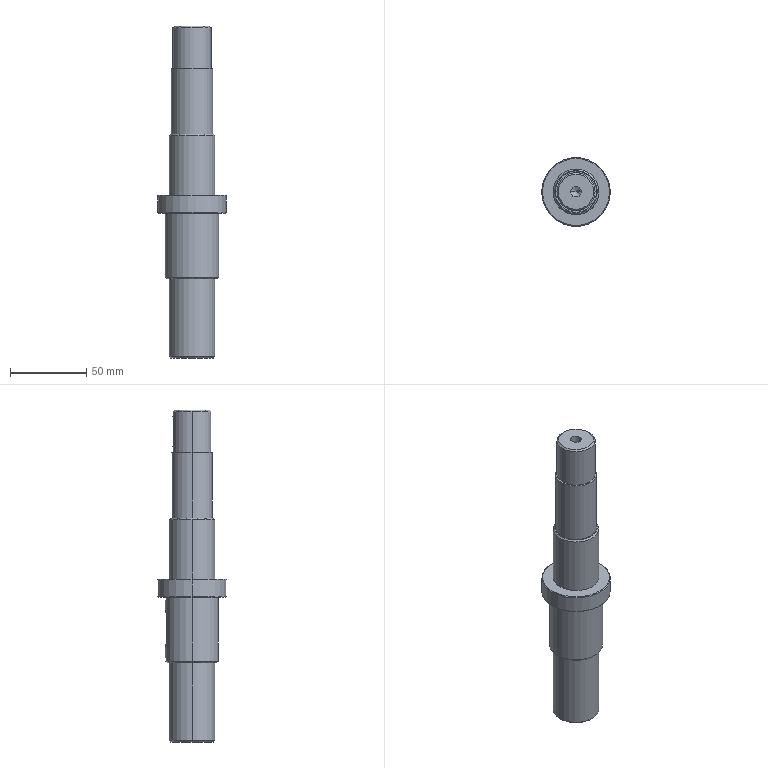Part | SolidWorks | features ICE 7, Chamfer 3, 3DProfileFeature 1, Extrusion 1, HoleWzd 1 | 1 solid | 47 faces | box 45 x 45 x 218 mm | volume 161225 mm3 | cylinder 20 | cone 14 | plane 13 | commonest cylinder face diameters 30 x4 8 x3 10 x3 7 x2 25 x2 27 x2
STEP:
#1=CARTESIAN_POINT('',(-3.5,0.,199.));
#2=VERTEX_POINT('',#1);
#3=CARTESIAN_POINT('',(3.5,0.,199.));
#4=VERTEX_POINT('',#3);
#5=CARTESIAN_POINT('',(0.,0.,199.));
#6=DIRECTION('',(0.,0.,1.));
#7=DIRECTION('',(1.,0.,0.));
#8=AXIS2_PLACEMENT_3D('',#5,#6,#7);
#9=CIRCLE('',#8,3.5);
#10=EDGE_CURVE('',#2,#4,#9,.T.);
#11=ORIENTED_EDGE('',*,*,#10,.F.);
#12=CARTESIAN_POINT('',(-3.5,0.,218.));
#13=VERTEX_POINT('',#12);
#14=CARTESIAN_POINT('',(-3.5,0.,218.));
#15=DIRECTION('',(0.,0.,1.));
#16=VECTOR('',#15,1000.);
#17=LINE('',#14,#16);
#18=EDGE_CURVE('',#2,#13,#17,.T.);
#19=ORIENTED_EDGE('',*,*,#18,.T.);
#20=CARTESIAN_POINT('',(3.5,0.,218.));
#21=VERTEX_POINT('',#20);
#22=CARTESIAN_POINT('',(0.,0.,218.));
#23=DIRECTION('',(0.,0.,1.));
#24=DIRECTION('',(1.,0.,0.));
#25=AXIS2_PLACEMENT_3D('',#22,#23,#24);
#26=CIRCLE('',#25,3.5);
#27=EDGE_CURVE('',#13,#21,#26,.T.);
#28=ORIENTED_EDGE('',*,*,#27,.T.);
#29=CARTESIAN_POINT('',(3.5,0.,218.));
#30=DIRECTION('',(0.,0.,1.));
#31=VECTOR('',#30,1000.);
#32=LINE('',#29,#31);
#33=EDGE_CURVE('',#4,#21,#32,.T.);
#34=ORIENTED_EDGE('',*,*,#33,.F.);
#35=EDGE_LOOP('',(#11,#19,#28,#34));
#36=FACE_OUTER_BOUND('',#35,.T.);
#37=CARTESIAN_POINT('',(0.,0.,218.));
#38=DIRECTION('',(0.,0.,1.));
#39=DIRECTION('',(1.,0.,0.));
#40=AXIS2_PLACEMENT_3D('',#37,#38,#39);
#41=CYLINDRICAL_SURFACE('',#40,3.5);
#42=ADVANCED_FACE('',(#36),#41,.F.);
#43=CARTESIAN_POINT('',(0.,0.,196.897));
#44=VERTEX_POINT('',#43);
#45=CARTESIAN_POINT('',(3.5,0.,199.));
#46=DIRECTION('',(0.8572,0.,0.515));
#47=VECTOR('',#46,1000.);
#48=LINE('',#45,#47);
#49=EDGE_CURVE('',#44,#4,#48,.T.);
#50=ORIENTED_EDGE('',*,*,#49,.F.);
#51=CARTESIAN_POINT('',(-3.5,0.,199.));
#52=DIRECTION('',(-0.8572,0.,0.515));
#53=VECTOR('',#52,1000.);
#54=LINE('',#51,#53);
#55=EDGE_CURVE('',#44,#2,#54,.T.);
#56=ORIENTED_EDGE('',*,*,#55,.T.);
#57=ORIENTED_EDGE('',*,*,#10,.T.);
#58=EDGE_LOOP('',(#50,#56,#57));
#59=FACE_OUTER_BOUND('',#58,.T.);
#60=CARTESIAN_POINT('',(0.,0.,199.));
#61=DIRECTION('',(0.,0.,1.));
#62=DIRECTION('',(1.,0.,0.));
#63=AXIS2_PLACEMENT_3D('',#60,#61,#62);
#64=CONICAL_SURFACE('',#63,3.5,1.03);
#65=ADVANCED_FACE('',(#59),#64,.F.);
#66=CARTESIAN_POINT('',(4.,11.843,198.));
#67=VERTEX_POINT('',#66);
#68=CARTESIAN_POINT('',(0.,12.5,194.));
#69=VERTEX_POINT('',#68);
#70=CARTESIAN_POINT('',(4.,11.843,198.));
#71=CARTESIAN_POINT('',(4.,11.843,197.734));
#72=CARTESIAN_POINT('',(3.974,11.852,197.472));
#73=CARTESIAN_POINT('',(3.871,11.886,196.959));
#74=CARTESIAN_POINT('',(3.793,11.911,196.704));
#75=CARTESIAN_POINT('',(3.592,11.973,196.22));
#76=CARTESIAN_POINT('',(3.469,12.01,195.991));
#77=CARTESIAN_POINT('',(3.178,12.09,195.557));
#78=CARTESIAN_POINT('',(3.011,12.134,195.354));
#79=CARTESIAN_POINT('',(2.644,12.219,194.987));
#80=CARTESIAN_POINT('',(2.444,12.261,194.822));
#81=CARTESIAN_POINT('',(2.006,12.34,194.53));
#82=CARTESIAN_POINT('',(1.776,12.375,194.407));
#83=CARTESIAN_POINT('',(1.295,12.435,194.207));
#84=CARTESIAN_POINT('',(1.041,12.459,194.129));
#85=CARTESIAN_POINT('',(0.5239,12.492,194.026));
#86=CARTESIAN_POINT('',(0.263,12.5,194.));
#87=CARTESIAN_POINT('',(0.,12.5,194.));
#88=B_SPLINE_CURVE_WITH_KNOTS('',3,(#70,#71,#72,#73,#74,#75,#76,#77,#78,#79,#80,#81,#82,#83,#84,#85,#86,#87),.UNSPECIFIED.,.F.,.F.,(4,2,2,2,2,2,2,2,4),(0.,0.000787,0.001574,0.002361,0.003148,0.003935,0.004722,0.005509,0.006296),.UNSPECIFIED.);
#89=EDGE_CURVE('',#67,#69,#88,.T.);
#90=ORIENTED_EDGE('',*,*,#89,.T.);
#91=CARTESIAN_POINT('',(0.,8.5,194.));
#92=VERTEX_POINT('',#91);
#93=CARTESIAN_POINT('',(0.,18.5,194.));
#94=DIRECTION('',(0.,-1.,0.));
#95=VECTOR('',#94,1000.);
#96=LINE('',#93,#95);
#97=EDGE_CURVE('',#69,#92,#96,.T.);
#98=ORIENTED_EDGE('',*,*,#97,.T.);
#99=CARTESIAN_POINT('',(4.,8.5,198.));
#100=VERTEX_POINT('',#99);
#101=CARTESIAN_POINT('',(0.,8.5,198.));
#102=DIRECTION('',(0.,1.,0.));
#103=DIRECTION('',(0.,0.,1.));
#104=AXIS2_PLACEMENT_3D('',#101,#102,#103);
#105=CIRCLE('',#104,4.);
#106=EDGE_CURVE('',#100,#92,#105,.T.);
#107=ORIENTED_EDGE('',*,*,#106,.F.);
#108=CARTESIAN_POINT('',(4.,18.5,198.));
#109=DIRECTION('',(0.,-1.,0.));
#110=VECTOR('',#109,1000.);
#111=LINE('',#108,#110);
#112=EDGE_CURVE('',#67,#100,#111,.T.);
#113=ORIENTED_EDGE('',*,*,#112,.F.);
#114=EDGE_LOOP('',(#90,#98,#107,#113));
#115=FACE_OUTER_BOUND('',#114,.T.);
#116=CARTESIAN_POINT('',(0.,18.5,198.));
#117=DIRECTION('',(0.,-1.,0.));
#118=DIRECTION('',(0.,0.,-1.));
#119=AXIS2_PLACEMENT_3D('',#116,#117,#118);
#120=CYLINDRICAL_SURFACE('',#119,4.);
#121=ADVANCED_FACE('',(#115),#120,.F.);
#122=CARTESIAN_POINT('',(5.,16.771,67.));
#123=VERTEX_POINT('',#122);
#124=CARTESIAN_POINT('',(0.,17.5,62.));
#125=VERTEX_POINT('',#124);
#126=CARTESIAN_POINT('',(5.,16.771,67.));
#127=CARTESIAN_POINT('',(5.,16.771,66.668));
#128=CARTESIAN_POINT('',(4.967,16.78,66.341));
#129=CARTESIAN_POINT('',(4.839,16.818,65.7));
#130=CARTESIAN_POINT('',(4.742,16.846,65.381));
#131=CARTESIAN_POINT('',(4.49,16.915,64.776));
#132=CARTESIAN_POINT('',(4.337,16.955,64.49));
#133=CARTESIAN_POINT('',(3.974,17.044,63.948));
#134=CARTESIAN_POINT('',(3.764,17.092,63.692));
#135=CARTESIAN_POINT('',(3.305,17.187,63.234));
#136=CARTESIAN_POINT('',(3.054,17.234,63.027));
#137=CARTESIAN_POINT('',(2.507,17.322,62.662));
#138=CARTESIAN_POINT('',(2.219,17.361,62.508));
#139=CARTESIAN_POINT('',(1.768,17.411,62.32));
#140=CARTESIAN_POINT('',(1.614,17.426,62.265));
#141=CARTESIAN_POINT('',(1.3,17.452,62.169));
#142=CARTESIAN_POINT('',(1.139,17.464,62.129));
#143=CARTESIAN_POINT('',(0.6539,17.491,62.032));
#144=CARTESIAN_POINT('',(0.3282,17.5,62.));
#145=CARTESIAN_POINT('',(0.,17.5,62.));
#146=B_SPLINE_CURVE_WITH_KNOTS('',3,(#126,#127,#128,#129,#130,#131,#132,#133,#134,#135,#136,#137,#138,#139,#140,#141,#142,#143,#144,#145),.UNSPECIFIED.,.F.,.F.,(4,2,2,2,2,2,2,2,2,4),(0.,0.0009824,0.001965,0.002947,0.00393,0.004912,0.005894,0.006386,0.006877,0.007859),.UNSPECIFIED.);
#147=EDGE_CURVE('',#123,#125,#146,.T.);
#148=ORIENTED_EDGE('',*,*,#147,.T.);
#149=CARTESIAN_POINT('',(0.,12.5,62.));
#150=VERTEX_POINT('',#149);
#151=CARTESIAN_POINT('',(0.,32.5,62.));
#152=DIRECTION('',(0.,-1.,0.));
#153=VECTOR('',#152,1000.);
#154=LINE('',#151,#153);
#155=EDGE_CURVE('',#125,#150,#154,.T.);
#156=ORIENTED_EDGE('',*,*,#155,.T.);
#157=CARTESIAN_POINT('',(5.,12.5,67.));
#158=VERTEX_POINT('',#157);
#159=CARTESIAN_POINT('',(0.,12.5,67.));
#160=DIRECTION('',(0.,1.,0.));
#161=DIRECTION('',(0.,0.,1.));
#162=AXIS2_PLACEMENT_3D('',#159,#160,#161);
#163=CIRCLE('',#162,5.);
#164=EDGE_CURVE('',#158,#150,#163,.T.);
#165=ORIENTED_EDGE('',*,*,#164,.F.);
#166=CARTESIAN_POINT('',(5.,32.5,67.));
#167=DIRECTION('',(0.,-1.,0.));
#168=VECTOR('',#167,1000.);
#169=LINE('',#166,#168);
#170=EDGE_CURVE('',#123,#158,#169,.T.);
#171=ORIENTED_EDGE('',*,*,#170,.F.);
#172=EDGE_LOOP('',(#148,#156,#165,#171));
#173=FACE_OUTER_BOUND('',#172,.T.);
#174=CARTESIAN_POINT('',(0.,32.5,67.));
#175=DIRECTION('',(0.,-1.,0.));
#176=DIRECTION('',(0.,0.,-1.));
#177=AXIS2_PLACEMENT_3D('',#174,#175,#176);
#178=CYLINDRICAL_SURFACE('',#177,5.);
#179=ADVANCED_FACE('',(#173),#178,.F.);
#180=CARTESIAN_POINT('',(-22.,0.,95.));
#181=VERTEX_POINT('',#180);
#182=CARTESIAN_POINT('',(22.,0.,95.));
#183=VERTEX_POINT('',#182);
#184=CARTESIAN_POINT('',(0.,0.,95.));
#185=DIRECTION('',(0.,0.,-1.));
#186=DIRECTION('',(1.,0.,0.));
#187=AXIS2_PLACEMENT_3D('',#184,#185,#186);
#188=CIRCLE('',#187,22.);
#189=EDGE_CURVE('',#181,#183,#188,.T.);
#190=ORIENTED_EDGE('',*,*,#189,.F.);
#191=CARTESIAN_POINT('',(-22.5,0.,95.5));
#192=VERTEX_POINT('',#191);
#193=CARTESIAN_POINT('',(-22.5,0.,95.5));
#194=DIRECTION('',(-0.7071,0.,0.7071));
#195=VECTOR('',#194,1000.);
#196=LINE('',#193,#195);
#197=EDGE_CURVE('',#181,#192,#196,.T.);
#198=ORIENTED_EDGE('',*,*,#197,.T.);
#199=CARTESIAN_POINT('',(22.5,0.,95.5));
#200=VERTEX_POINT('',#199);
#201=CARTESIAN_POINT('',(0.,0.,95.5));
#202=DIRECTION('',(0.,0.,1.));
#203=DIRECTION('',(1.,0.,0.));
#204=AXIS2_PLACEMENT_3D('',#201,#202,#203);
#205=CIRCLE('',#204,22.5);
#206=EDGE_CURVE('',#200,#192,#205,.T.);
#207=ORIENTED_EDGE('',*,*,#206,.F.);
#208=CARTESIAN_POINT('',(22.5,0.,95.5));
#209=DIRECTION('',(0.7071,0.,0.7071));
#210=VECTOR('',#209,1000.);
#211=LINE('',#208,#210);
#212=EDGE_CURVE('',#183,#200,#211,.T.);
#213=ORIENTED_EDGE('',*,*,#212,.F.);
#214=EDGE_LOOP('',(#190,#198,#207,#213));
#215=FACE_OUTER_BOUND('',#214,.T.);
#216=CARTESIAN_POINT('',(0.,0.,95.5));
#217=DIRECTION('',(0.,0.,1.));
#218=DIRECTION('',(1.,0.,0.));
#219=AXIS2_PLACEMENT_3D('',#216,#217,#218);
#220=CONICAL_SURFACE('',#219,22.5,0.7854);
#221=ADVANCED_FACE('',(#215),#220,.T.);
#222=CARTESIAN_POINT('',(22.,0.,107.));
#223=VERTEX_POINT('',#222);
#224=CARTESIAN_POINT('',(-22.,0.,107.));
#225=VERTEX_POINT('',#224);
#226=CARTESIAN_POINT('',(0.,0.,107.));
#227=DIRECTION('',(0.,0.,1.));
#228=DIRECTION('',(1.,0.,0.));
#229=AXIS2_PLACEMENT_3D('',#226,#227,#228);
#230=CIRCLE('',#229,22.);
#231=EDGE_CURVE('',#223,#225,#230,.T.);
#232=ORIENTED_EDGE('',*,*,#231,.F.);
#233=CARTESIAN_POINT('',(22.5,0.,106.5));
#234=VERTEX_POINT('',#233);
#235=CARTESIAN_POINT('',(22.,0.,107.));
#236=DIRECTION('',(0.7071,0.,-0.7071));
#237=VECTOR('',#236,1000.);
#238=LINE('',#235,#237);
#239=EDGE_CURVE('',#223,#234,#238,.T.);
#240=ORIENTED_EDGE('',*,*,#239,.T.);
#241=CARTESIAN_POINT('',(-22.5,0.,106.5));
#242=VERTEX_POINT('',#241);
#243=CARTESIAN_POINT('',(0.,0.,106.5));
#244=DIRECTION('',(0.,0.,-1.));
#245=DIRECTION('',(1.,0.,0.));
#246=AXIS2_PLACEMENT_3D('',#243,#244,#245);
#247=CIRCLE('',#246,22.5);
#248=EDGE_CURVE('',#242,#234,#247,.T.);
#249=ORIENTED_EDGE('',*,*,#248,.F.);
#250=CARTESIAN_POINT('',(-22.,0.,107.));
#251=DIRECTION('',(-0.7071,0.,-0.7071));
#252=VECTOR('',#251,1000.);
#253=LINE('',#250,#252);
#254=EDGE_CURVE('',#225,#242,#253,.T.);
#255=ORIENTED_EDGE('',*,*,#254,.F.);
#256=EDGE_LOOP('',(#232,#240,#249,#255));
#257=FACE_OUTER_BOUND('',#256,.T.);
#258=CARTESIAN_POINT('',(0.,0.,107.));
#259=DIRECTION('',(0.,0.,-1.));
#260=DIRECTION('',(-1.,0.,0.));
#261=AXIS2_PLACEMENT_3D('',#258,#259,#260);
#262=CONICAL_SURFACE('',#261,22.,0.7854);
#263=ADVANCED_FACE('',(#257),#262,.T.);
#264=CARTESIAN_POINT('',(-16.5,0.,52.));
#265=VERTEX_POINT('',#264);
#266=CARTESIAN_POINT('',(16.5,0.,52.));
#267=VERTEX_POINT('',#266);
#268=CARTESIAN_POINT('',(0.,0.,52.));
#269=DIRECTION('',(0.,0.,-1.));
#270=DIRECTION('',(1.,0.,0.));
#271=AXIS2_PLACEMENT_3D('',#268,#269,#270);
#272=CIRCLE('',#271,16.5);
#273=EDGE_CURVE('',#265,#267,#272,.T.);
#274=ORIENTED_EDGE('',*,*,#273,.F.);
#275=CARTESIAN_POINT('',(-17.5,0.,53.));
#276=VERTEX_POINT('',#275);
#277=CARTESIAN_POINT('',(-17.5,0.,53.));
#278=DIRECTION('',(-0.7071,0.,0.7071));
#279=VECTOR('',#278,1000.);
#280=LINE('',#277,#279);
#281=EDGE_CURVE('',#265,#276,#280,.T.);
#282=ORIENTED_EDGE('',*,*,#281,.T.);
#283=CARTESIAN_POINT('',(17.5,0.,53.));
#284=VERTEX_POINT('',#283);
#285=CARTESIAN_POINT('',(0.,0.,53.));
#286=DIRECTION('',(0.,0.,1.));
#287=DIRECTION('',(1.,0.,0.));
#288=AXIS2_PLACEMENT_3D('',#285,#286,#287);
#289=CIRCLE('',#288,17.5);
#290=EDGE_CURVE('',#284,#276,#289,.T.);
#291=ORIENTED_EDGE('',*,*,#290,.F.);
#292=CARTESIAN_POINT('',(17.5,0.,53.));
#293=DIRECTION('',(0.7071,0.,0.7071));
#294=VECTOR('',#293,1000.);
#295=LINE('',#292,#294);
#296=EDGE_CURVE('',#267,#284,#295,.T.);
#297=ORIENTED_EDGE('',*,*,#296,.F.);
#298=EDGE_LOOP('',(#274,#282,#291,#297));
#299=FACE_OUTER_BOUND('',#298,.T.);
#300=CARTESIAN_POINT('',(0.,0.,53.));
#301=DIRECTION('',(0.,0.,1.));
#302=DIRECTION('',(1.,0.,0.));
#303=AXIS2_PLACEMENT_3D('',#300,#301,#302);
#304=CONICAL_SURFACE('',#303,17.5,0.7854);
#305=ADVANCED_FACE('',(#299),#304,.T.);
#306=CARTESIAN_POINT('',(14.,0.,147.));
#307=VERTEX_POINT('',#306);
#308=CARTESIAN_POINT('',(-14.,0.,147.));
#309=VERTEX_POINT('',#308);
#310=CARTESIAN_POINT('',(0.,0.,147.));
#311=DIRECTION('',(0.,0.,1.));
#312=DIRECTION('',(1.,0.,0.));
#313=AXIS2_PLACEMENT_3D('',#310,#311,#312);
#314=CIRCLE('',#313,14.);
#315=EDGE_CURVE('',#307,#309,#314,.T.);
#316=ORIENTED_EDGE('',*,*,#315,.F.);
#317=CARTESIAN_POINT('',(15.,0.,146.));
#318=VERTEX_POINT('',#317);
#319=CARTESIAN_POINT('',(14.,0.,147.));
#320=DIRECTION('',(0.7071,0.,-0.7071));
#321=VECTOR('',#320,1000.);
#322=LINE('',#319,#321);
#323=EDGE_CURVE('',#307,#318,#322,.T.);
#324=ORIENTED_EDGE('',*,*,#323,.T.);
#325=CARTESIAN_POINT('',(-15.,0.,146.));
#326=VERTEX_POINT('',#325);
#327=CARTESIAN_POINT('',(0.,0.,146.));
#328=DIRECTION('',(0.,0.,-1.));
#329=DIRECTION('',(1.,0.,0.));
#330=AXIS2_PLACEMENT_3D('',#327,#328,#329);
#331=CIRCLE('',#330,15.);
#332=EDGE_CURVE('',#326,#318,#331,.T.);
#333=ORIENTED_EDGE('',*,*,#332,.F.);
#334=CARTESIAN_POINT('',(-14.,0.,147.));
#335=DIRECTION('',(-0.7071,0.,-0.7071));
#336=VECTOR('',#335,1000.);
#337=LINE('',#334,#336);
#338=EDGE_CURVE('',#309,#326,#337,.T.);
#339=ORIENTED_EDGE('',*,*,#338,.F.);
#340=EDGE_LOOP('',(#316,#324,#333,#339));
#341=FACE_OUTER_BOUND('',#340,.T.);
#342=CARTESIAN_POINT('',(0.,0.,147.));
#343=DIRECTION('',(0.,0.,-1.));
#344=DIRECTION('',(-1.,0.,0.));
#345=AXIS2_PLACEMENT_3D('',#342,#343,#344);
#346=CONICAL_SURFACE('',#345,14.,0.7854);
#347=ADVANCED_FACE('',(#341),#346,.T.);
#348=CARTESIAN_POINT('',(11.5,0.,218.));
#349=VERTEX_POINT('',#348);
#350=CARTESIAN_POINT('',(-11.5,0.,218.));
#351=VERTEX_POINT('',#350);
#352=CARTESIAN_POINT('',(0.,0.,218.));
#353=DIRECTION('',(0.,0.,1.));
#354=DIRECTION('',(1.,0.,0.));
#355=AXIS2_PLACEMENT_3D('',#352,#353,#354);
#356=CIRCLE('',#355,11.5);
#357=EDGE_CURVE('',#349,#351,#356,.T.);
#358=ORIENTED_EDGE('',*,*,#357,.F.);
#359=CARTESIAN_POINT('',(12.5,0.,217.));
#360=VERTEX_POINT('',#359);
#361=CARTESIAN_POINT('',(11.5,0.,218.));
#362=DIRECTION('',(0.7071,0.,-0.7071));
#363=VECTOR('',#362,1000.);
#364=LINE('',#361,#363);
#365=EDGE_CURVE('',#349,#360,#364,.T.);
#366=ORIENTED_EDGE('',*,*,#365,.T.);
#367=CARTESIAN_POINT('',(-12.5,0.,217.));
#368=VERTEX_POINT('',#367);
#369=CARTESIAN_POINT('',(0.,0.,217.));
#370=DIRECTION('',(0.,0.,-1.));
#371=DIRECTION('',(1.,0.,0.));
#372=AXIS2_PLACEMENT_3D('',#369,#370,#371);
#373=CIRCLE('',#372,12.5);
#374=EDGE_CURVE('',#368,#360,#373,.T.);
#375=ORIENTED_EDGE('',*,*,#374,.F.);
#376=CARTESIAN_POINT('',(-11.5,0.,218.));
#377=DIRECTION('',(-0.7071,0.,-0.7071));
#378=VECTOR('',#377,1000.);
#379=LINE('',#376,#378);
#380=EDGE_CURVE('',#351,#368,#379,.T.);
#381=ORIENTED_EDGE('',*,*,#380,.F.);
#382=EDGE_LOOP('',(#358,#366,#375,#381));
#383=FACE_OUTER_BOUND('',#382,.T.);
#384=CARTESIAN_POINT('',(0.,0.,218.));
#385=DIRECTION('',(0.,0.,-1.));
#386=DIRECTION('',(-1.,0.,0.));
#387=AXIS2_PLACEMENT_3D('',#384,#385,#386);
#388=CONICAL_SURFACE('',#387,11.5,0.7854);
#389=ADVANCED_FACE('',(#383),#388,.T.);
#390=CARTESIAN_POINT('',(-14.,0.,0.));
#391=VERTEX_POINT('',#390);
#392=CARTESIAN_POINT('',(14.,0.,0.));
#393=VERTEX_POINT('',#392);
#394=CARTESIAN_POINT('',(0.,0.,0.));
#395=DIRECTION('',(0.,0.,-1.));
#396=DIRECTION('',(1.,0.,0.));
#397=AXIS2_PLACEMENT_3D('',#394,#395,#396);
#398=CIRCLE('',#397,14.);
#399=EDGE_CURVE('',#391,#393,#398,.T.);
#400=ORIENTED_EDGE('',*,*,#399,.F.);
#401=CARTESIAN_POINT('',(-15.,0.,1.));
#402=VERTEX_POINT('',#401);
#403=CARTESIAN_POINT('',(-15.,0.,1.));
#404=DIRECTION('',(-0.7071,0.,0.7071));
#405=VECTOR('',#404,1000.);
#406=LINE('',#403,#405);
#407=EDGE_CURVE('',#391,#402,#406,.T.);
#408=ORIENTED_EDGE('',*,*,#407,.T.);
#409=CARTESIAN_POINT('',(15.,0.,1.));
#410=VERTEX_POINT('',#409);
#411=CARTESIAN_POINT('',(0.,0.,1.));
#412=DIRECTION('',(0.,0.,1.));
#413=DIRECTION('',(1.,0.,0.));
#414=AXIS2_PLACEMENT_3D('',#411,#412,#413);
#415=CIRCLE('',#414,15.);
#416=EDGE_CURVE('',#410,#402,#415,.T.);
#417=ORIENTED_EDGE('',*,*,#416,.F.);
#418=CARTESIAN_POINT('',(15.,0.,1.));
#419=DIRECTION('',(0.7071,0.,0.7071));
#420=VECTOR('',#419,1000.);
#421=LINE('',#418,#420);
#422=EDGE_CURVE('',#393,#410,#421,.T.);
#423=ORIENTED_EDGE('',*,*,#422,.F.);
#424=EDGE_LOOP('',(#400,#408,#417,#423));
#425=FACE_OUTER_BOUND('',#424,.T.);
#426=CARTESIAN_POINT('',(0.,0.,1.));
#427=DIRECTION('',(0.,0.,1.));
#428=DIRECTION('',(1.,0.,0.));
#429=AXIS2_PLACEMENT_3D('',#426,#427,#428);
#430=CONICAL_SURFACE('',#429,15.,0.7854);
#431=ADVANCED_FACE('',(#425),#430,.T.);
#432=CARTESIAN_POINT('',(13.5,0.,190.));
#433=VERTEX_POINT('',#432);
#434=CARTESIAN_POINT('',(-13.5,0.,190.));
#435=VERTEX_POINT('',#434);
#436=CARTESIAN_POINT('',(0.,0.,190.));
#437=DIRECTION('',(0.,0.,1.));
#438=DIRECTION('',(1.,0.,0.));
#439=AXIS2_PLACEMENT_3D('',#436,#437,#438);
#440=CIRCLE('',#439,13.5);
#441=EDGE_CURVE('',#433,#435,#440,.T.);
#442=ORIENTED_EDGE('',*,*,#441,.F.);
#443=CARTESIAN_POINT('',(13.5,0.,147.));
#444=VERTEX_POINT('',#443);
#445=CARTESIAN_POINT('',(13.5,0.,190.));
#446=DIRECTION('',(0.,0.,-1.));
#447=VECTOR('',#446,1000.);
#448=LINE('',#445,#447);
#449=EDGE_CURVE('',#433,#444,#448,.T.);
#450=ORIENTED_EDGE('',*,*,#449,.T.);
#451=CARTESIAN_POINT('',(-13.5,0.,147.));
#452=VERTEX_POINT('',#451);
#453=CARTESIAN_POINT('',(0.,0.,147.));
#454=DIRECTION('',(0.,0.,1.));
#455=DIRECTION('',(1.,0.,0.));
#456=AXIS2_PLACEMENT_3D('',#453,#454,#455);
#457=CIRCLE('',#456,13.5);
#458=EDGE_CURVE('',#444,#452,#457,.T.);
#459=ORIENTED_EDGE('',*,*,#458,.T.);
#460=CARTESIAN_POINT('',(-13.5,0.,190.));
#461=DIRECTION('',(0.,0.,-1.));
#462=VECTOR('',#461,1000.);
#463=LINE('',#460,#462);
#464=EDGE_CURVE('',#435,#452,#463,.T.);
#465=ORIENTED_EDGE('',*,*,#464,.F.);
#466=EDGE_LOOP('',(#442,#450,#459,#465));
#467=FACE_OUTER_BOUND('',#466,.T.);
#468=CARTESIAN_POINT('',(0.,0.,190.));
#469=DIRECTION('',(0.,0.,-1.));
#470=DIRECTION('',(-1.,0.,0.));
#471=AXIS2_PLACEMENT_3D('',#468,#469,#470);
#472=CYLINDRICAL_SURFACE('',#471,13.5);
#473=ADVANCED_FACE('',(#467),#472,.T.);
#474=ORIENTED_EDGE('',*,*,#332,.T.);
#475=CARTESIAN_POINT('',(15.,0.,107.));
#476=VERTEX_POINT('',#475);
#477=CARTESIAN_POINT('',(15.,0.,147.));
#478=DIRECTION('',(0.,0.,-1.));
#479=VECTOR('',#478,1000.);
#480=LINE('',#477,#479);
#481=EDGE_CURVE('',#318,#476,#480,.T.);
#482=ORIENTED_EDGE('',*,*,#481,.T.);
#483=CARTESIAN_POINT('',(-15.,0.,107.));
#484=VERTEX_POINT('',#483);
#485=CARTESIAN_POINT('',(0.,0.,107.));
#486=DIRECTION('',(0.,0.,1.));
#487=DIRECTION('',(1.,0.,0.));
#488=AXIS2_PLACEMENT_3D('',#485,#486,#487);
#489=CIRCLE('',#488,15.);
#490=EDGE_CURVE('',#476,#484,#489,.T.);
#491=ORIENTED_EDGE('',*,*,#490,.T.);
#492=CARTESIAN_POINT('',(-15.,0.,147.));
#493=DIRECTION('',(0.,0.,-1.));
#494=VECTOR('',#493,1000.);
#495=LINE('',#492,#494);
#496=EDGE_CURVE('',#326,#484,#495,.T.);
#497=ORIENTED_EDGE('',*,*,#496,.F.);
#498=EDGE_LOOP('',(#474,#482,#491,#497));
#499=FACE_OUTER_BOUND('',#498,.T.);
#500=CARTESIAN_POINT('',(0.,0.,147.));
#501=DIRECTION('',(0.,0.,-1.));
#502=DIRECTION('',(-1.,0.,0.));
#503=AXIS2_PLACEMENT_3D('',#500,#501,#502);
#504=CYLINDRICAL_SURFACE('',#503,15.);
#505=ADVANCED_FACE('',(#499),#504,.T.);
#506=ORIENTED_EDGE('',*,*,#248,.T.);
#507=CARTESIAN_POINT('',(22.5,0.,107.));
#508=DIRECTION('',(0.,0.,-1.));
#509=VECTOR('',#508,1000.);
#510=LINE('',#507,#509);
#511=EDGE_CURVE('',#234,#200,#510,.T.);
#512=ORIENTED_EDGE('',*,*,#511,.T.);
#513=ORIENTED_EDGE('',*,*,#206,.T.);
#514=CARTESIAN_POINT('',(-22.5,0.,107.));
#515=DIRECTION('',(0.,0.,-1.));
#516=VECTOR('',#515,1000.);
#517=LINE('',#514,#516);
#518=EDGE_CURVE('',#242,#192,#517,.T.);
#519=ORIENTED_EDGE('',*,*,#518,.F.);
#520=EDGE_LOOP('',(#506,#512,#513,#519));
#521=FACE_OUTER_BOUND('',#520,.T.);
#522=CARTESIAN_POINT('',(0.,0.,107.));
#523=DIRECTION('',(0.,0.,-1.));
#524=DIRECTION('',(-1.,0.,0.));
#525=AXIS2_PLACEMENT_3D('',#522,#523,#524);
#526=CYLINDRICAL_SURFACE('',#525,22.5);
#527=ADVANCED_FACE('',(#521),#526,.T.);
#528=CARTESIAN_POINT('',(15.,0.,52.));
#529=VERTEX_POINT('',#528);
#530=CARTESIAN_POINT('',(-15.,0.,52.));
#531=VERTEX_POINT('',#530);
#532=CARTESIAN_POINT('',(0.,0.,52.));
#533=DIRECTION('',(0.,0.,1.));
#534=DIRECTION('',(1.,0.,0.));
#535=AXIS2_PLACEMENT_3D('',#532,#533,#534);
#536=CIRCLE('',#535,15.);
#537=EDGE_CURVE('',#529,#531,#536,.T.);
#538=ORIENTED_EDGE('',*,*,#537,.F.);
#539=CARTESIAN_POINT('',(15.,0.,52.));
#540=DIRECTION('',(0.,0.,-1.));
#541=VECTOR('',#540,1000.);
#542=LINE('',#539,#541);
#543=EDGE_CURVE('',#529,#410,#542,.T.);
#544=ORIENTED_EDGE('',*,*,#543,.T.);
#545=ORIENTED_EDGE('',*,*,#416,.T.);
#546=CARTESIAN_POINT('',(-15.,0.,52.));
#547=DIRECTION('',(0.,0.,-1.));
#548=VECTOR('',#547,1000.);
#549=LINE('',#546,#548);
#550=EDGE_CURVE('',#531,#402,#549,.T.);
#551=ORIENTED_EDGE('',*,*,#550,.F.);
#552=EDGE_LOOP('',(#538,#544,#545,#551));
#553=FACE_OUTER_BOUND('',#552,.T.);
#554=CARTESIAN_POINT('',(0.,0.,52.));
#555=DIRECTION('',(0.,0.,-1.));
#556=DIRECTION('',(-1.,0.,0.));
#557=AXIS2_PLACEMENT_3D('',#554,#555,#556);
#558=CYLINDRICAL_SURFACE('',#557,15.);
#559=ADVANCED_FACE('',(#553),#558,.T.);
#560=ORIENTED_EDGE('',*,*,#147,.F.);
#561=CARTESIAN_POINT('',(5.,16.771,82.));
#562=VERTEX_POINT('',#561);
#563=CARTESIAN_POINT('',(5.,16.771,95.));
#564=DIRECTION('',(0.,0.,-1.));
#565=VECTOR('',#564,1000.);
#566=LINE('',#563,#565);
#567=EDGE_CURVE('',#562,#123,#566,.T.);
#568=ORIENTED_EDGE('',*,*,#567,.F.);
#569=CARTESIAN_POINT('',(-5.,16.771,82.));
#570=VERTEX_POINT('',#569);
#571=CARTESIAN_POINT('',(-5.,16.771,82.));
#572=CARTESIAN_POINT('',(-5.,16.771,82.332));
#573=CARTESIAN_POINT('',(-4.967,16.78,82.658));
#574=CARTESIAN_POINT('',(-4.839,16.818,83.3));
#575=CARTESIAN_POINT('',(-4.742,16.846,83.618));
#576=CARTESIAN_POINT('',(-4.491,16.914,84.222));
#577=CARTESIAN_POINT('',(-4.337,16.955,84.509));
#578=CARTESIAN_POINT('',(-3.975,17.044,85.051));
#579=CARTESIAN_POINT('',(-3.765,17.092,85.306));
#580=CARTESIAN_POINT('',(-3.306,17.186,85.765));
#581=CARTESIAN_POINT('',(-3.056,17.233,85.971));
#582=CARTESIAN_POINT('',(-2.51,17.321,86.337));
#583=CARTESIAN_POINT('',(-2.222,17.361,86.491));
#584=CARTESIAN_POINT('',(-1.771,17.411,86.679));
#585=CARTESIAN_POINT('',(-1.618,17.426,86.734));
#586=CARTESIAN_POINT('',(-1.304,17.452,86.83));
#587=CARTESIAN_POINT('',(-1.143,17.463,86.87));
#588=CARTESIAN_POINT('',(-0.6583,17.491,86.967));
#589=CARTESIAN_POINT('',(-0.3328,17.5,87.));
#590=CARTESIAN_POINT('',(0.3232,17.5,87.));
#591=CARTESIAN_POINT('',(0.6564,17.491,86.968));
#592=CARTESIAN_POINT('',(1.299,17.455,86.839));
#593=CARTESIAN_POINT('',(1.612,17.428,86.745));
#594=CARTESIAN_POINT('',(2.219,17.361,86.493));
#595=CARTESIAN_POINT('',(2.509,17.321,86.337));
#596=CARTESIAN_POINT('',(3.049,17.235,85.976));
#597=CARTESIAN_POINT('',(3.303,17.187,85.768));
#598=CARTESIAN_POINT('',(3.765,17.092,85.306));
#599=CARTESIAN_POINT('',(3.971,17.045,85.055));
#600=CARTESIAN_POINT('',(4.333,16.956,84.516));
#601=CARTESIAN_POINT('',(4.49,16.915,84.223));
#602=CARTESIAN_POINT('',(4.741,16.846,83.621));
#603=CARTESIAN_POINT('',(4.837,16.818,83.309));
#604=CARTESIAN_POINT('',(4.967,16.781,82.664));
#605=CARTESIAN_POINT('',(5.,16.771,82.332));
#606=CARTESIAN_POINT('',(5.,16.771,82.));
#607=B_SPLINE_CURVE_WITH_KNOTS('',3,(#571,#572,#573,#574,#575,#576,#577,#578,#579,#580,#581,#582,#583,#584,#585,#586,#587,#588,#589,#590,#591,#592,#593,#594,#595,#596,#597,#598,#599,#600,#601,#602,#603,#604,#605,#606),.UNSPECIFIED.,.F.,.F.,(4,2,2,2,2,2,2,2,2,2,2,2,2,2,2,2,2,4),(0.,0.0009818,0.001964,0.002945,0.003927,0.004909,0.005891,0.006382,0.006873,0.007855,0.008836,0.009818,0.0108,0.01178,0.01276,0.01375,0.01473,0.01571),.UNSPECIFIED.);
#608=EDGE_CURVE('',#570,#562,#607,.T.);
#609=ORIENTED_EDGE('',*,*,#608,.F.);
#610=CARTESIAN_POINT('',(-5.,16.771,67.));
#611=VERTEX_POINT('',#610);
#612=CARTESIAN_POINT('',(-5.,16.771,95.));
#613=DIRECTION('',(0.,0.,1.));
#614=VECTOR('',#613,1000.);
#615=LINE('',#612,#614);
#616=EDGE_CURVE('',#611,#570,#615,.T.);
#617=ORIENTED_EDGE('',*,*,#616,.F.);
#618=CARTESIAN_POINT('',(0.,17.5,62.));
#619=CARTESIAN_POINT('',(-0.3278,17.5,62.));
#620=CARTESIAN_POINT('',(-0.6608,17.49,62.033));
#621=CARTESIAN_POINT('',(-1.303,17.454,62.162));
#622=CARTESIAN_POINT('',(-1.615,17.428,62.257));
#623=CARTESIAN_POINT('',(-2.222,17.361,62.509));
#624=CARTESIAN_POINT('',(-2.512,17.321,62.665));
#625=CARTESIAN_POINT('',(-3.051,17.234,63.026));
#626=CARTESIAN_POINT('',(-3.305,17.187,63.234));
#627=CARTESIAN_POINT('',(-3.767,17.091,63.696));
#628=CARTESIAN_POINT('',(-3.972,17.044,63.946));
#629=CARTESIAN_POINT('',(-4.334,16.956,64.486));
#630=CARTESIAN_POINT('',(-4.491,16.914,64.778));
#631=CARTESIAN_POINT('',(-4.742,16.846,65.38));
#632=CARTESIAN_POINT('',(-4.837,16.818,65.692));
#633=CARTESIAN_POINT('',(-4.967,16.781,66.336));
#634=CARTESIAN_POINT('',(-5.,16.771,66.668));
#635=CARTESIAN_POINT('',(-5.,16.771,67.));
#636=B_SPLINE_CURVE_WITH_KNOTS('',3,(#618,#619,#620,#621,#622,#623,#624,#625,#626,#627,#628,#629,#630,#631,#632,#633,#634,#635),.UNSPECIFIED.,.F.,.F.,(4,2,2,2,2,2,2,2,4),(0.007859,0.008841,0.009822,0.0108,0.01178,0.01277,0.01375,0.01473,0.01571),.UNSPECIFIED.);
#637=EDGE_CURVE('',#125,#611,#636,.T.);
#638=ORIENTED_EDGE('',*,*,#637,.F.);
#639=EDGE_LOOP('',(#560,#568,#609,#617,#638));
#640=FACE_BOUND('',#639,.T.);
#641=CARTESIAN_POINT('',(17.5,0.,95.));
#642=VERTEX_POINT('',#641);
#643=CARTESIAN_POINT('',(-17.5,0.,95.));
#644=VERTEX_POINT('',#643);
#645=CARTESIAN_POINT('',(0.,0.,95.));
#646=DIRECTION('',(0.,0.,1.));
#647=DIRECTION('',(1.,0.,0.));
#648=AXIS2_PLACEMENT_3D('',#645,#646,#647);
#649=CIRCLE('',#648,17.5);
#650=EDGE_CURVE('',#642,#644,#649,.T.);
#651=ORIENTED_EDGE('',*,*,#650,.F.);
#652=CARTESIAN_POINT('',(17.5,0.,95.));
#653=DIRECTION('',(0.,0.,-1.));
#654=VECTOR('',#653,1000.);
#655=LINE('',#652,#654);
#656=EDGE_CURVE('',#642,#284,#655,.T.);
#657=ORIENTED_EDGE('',*,*,#656,.T.);
#658=ORIENTED_EDGE('',*,*,#290,.T.);
#659=CARTESIAN_POINT('',(-17.5,0.,95.));
#660=DIRECTION('',(0.,0.,-1.));
#661=VECTOR('',#660,1000.);
#662=LINE('',#659,#661);
#663=EDGE_CURVE('',#644,#276,#662,.T.);
#664=ORIENTED_EDGE('',*,*,#663,.F.);
#665=EDGE_LOOP('',(#651,#657,#658,#664));
#666=FACE_OUTER_BOUND('',#665,.T.);
#667=CARTESIAN_POINT('',(0.,0.,95.));
#668=DIRECTION('',(0.,0.,-1.));
#669=DIRECTION('',(-1.,0.,0.));
#670=AXIS2_PLACEMENT_3D('',#667,#668,#669);
#671=CYLINDRICAL_SURFACE('',#670,17.5);
#672=ADVANCED_FACE('',(#640,#666),#671,.T.);
#673=ORIENTED_EDGE('',*,*,#89,.F.);
#674=CARTESIAN_POINT('',(4.,11.843,210.));
#675=VERTEX_POINT('',#674);
#676=CARTESIAN_POINT('',(4.,11.843,218.));
#677=DIRECTION('',(0.,0.,-1.));
#678=VECTOR('',#677,1000.);
#679=LINE('',#676,#678);
#680=EDGE_CURVE('',#675,#67,#679,.T.);
#681=ORIENTED_EDGE('',*,*,#680,.F.);
#682=CARTESIAN_POINT('',(-4.,11.843,210.));
#683=VERTEX_POINT('',#682);
#684=CARTESIAN_POINT('',(-4.,11.843,210.));
#685=CARTESIAN_POINT('',(-4.,11.843,210.266));
#686=CARTESIAN_POINT('',(-3.974,11.852,210.527));
#687=CARTESIAN_POINT('',(-3.871,11.886,211.041));
#688=CARTESIAN_POINT('',(-3.793,11.911,211.296));
#689=CARTESIAN_POINT('',(-3.592,11.973,211.779));
#690=CARTESIAN_POINT('',(-3.469,12.01,212.008));
#691=CARTESIAN_POINT('',(-3.179,12.09,212.441));
#692=CARTESIAN_POINT('',(-3.012,12.133,212.645));
#693=CARTESIAN_POINT('',(-2.646,12.218,213.011));
#694=CARTESIAN_POINT('',(-2.445,12.26,213.176));
#695=CARTESIAN_POINT('',(-2.009,12.34,213.469));
#696=CARTESIAN_POINT('',(-1.779,12.375,213.592));
#697=CARTESIAN_POINT('',(-1.299,12.435,213.792));
#698=CARTESIAN_POINT('',(-1.045,12.459,213.87));
#699=CARTESIAN_POINT('',(-0.5276,12.492,213.974));
#700=CARTESIAN_POINT('',(-0.2669,12.5,214.));
#701=CARTESIAN_POINT('',(0.2587,12.5,214.));
#702=CARTESIAN_POINT('',(0.5256,12.492,213.974));
#703=CARTESIAN_POINT('',(1.04,12.459,213.871));
#704=CARTESIAN_POINT('',(1.29,12.436,213.795));
#705=CARTESIAN_POINT('',(1.777,12.375,213.593));
#706=CARTESIAN_POINT('',(2.008,12.34,213.469));
#707=CARTESIAN_POINT('',(2.44,12.262,213.18));
#708=CARTESIAN_POINT('',(2.643,12.219,213.013));
#709=CARTESIAN_POINT('',(3.012,12.133,212.645));
#710=CARTESIAN_POINT('',(3.176,12.091,212.445));
#711=CARTESIAN_POINT('',(3.466,12.011,212.013));
#712=CARTESIAN_POINT('',(3.592,11.973,211.78));
#713=CARTESIAN_POINT('',(3.792,11.911,211.298));
#714=CARTESIAN_POINT('',(3.869,11.886,211.049));
#715=CARTESIAN_POINT('',(3.973,11.852,210.532));
#716=CARTESIAN_POINT('',(4.,11.843,210.266));
#717=CARTESIAN_POINT('',(4.,11.843,210.));
#718=B_SPLINE_CURVE_WITH_KNOTS('',3,(#684,#685,#686,#687,#688,#689,#690,#691,#692,#693,#694,#695,#696,#697,#698,#699,#700,#701,#702,#703,#704,#705,#706,#707,#708,#709,#710,#711,#712,#713,#714,#715,#716,#717),.UNSPECIFIED.,.F.,.F.,(4,2,2,2,2,2,2,2,2,2,2,2,2,2,2,2,4),(0.,0.0007865,0.001573,0.00236,0.003146,0.003933,0.004719,0.005506,0.006292,0.007079,0.007865,0.008652,0.009438,0.01022,0.01101,0.0118,0.01258),.UNSPECIFIED.);
#719=EDGE_CURVE('',#683,#675,#718,.T.);
#720=ORIENTED_EDGE('',*,*,#719,.F.);
#721=CARTESIAN_POINT('',(-4.,11.843,198.));
#722=VERTEX_POINT('',#721);
#723=CARTESIAN_POINT('',(-4.,11.843,218.));
#724=DIRECTION('',(0.,0.,1.));
#725=VECTOR('',#724,1000.);
#726=LINE('',#723,#725);
#727=EDGE_CURVE('',#722,#683,#726,.T.);
#728=ORIENTED_EDGE('',*,*,#727,.F.);
#729=CARTESIAN_POINT('',(0.,12.5,194.));
#730=CARTESIAN_POINT('',(-0.2627,12.5,194.));
#731=CARTESIAN_POINT('',(-0.5294,12.491,194.027));
#732=CARTESIAN_POINT('',(-1.043,12.459,194.13));
#733=CARTESIAN_POINT('',(-1.293,12.435,194.206));
#734=CARTESIAN_POINT('',(-1.78,12.375,194.408));
#735=CARTESIAN_POINT('',(-2.011,12.339,194.532));
#736=CARTESIAN_POINT('',(-2.442,12.261,194.821));
#737=CARTESIAN_POINT('',(-2.645,12.218,194.988));
#738=CARTESIAN_POINT('',(-3.013,12.133,195.356));
#739=CARTESIAN_POINT('',(-3.177,12.09,195.556));
#740=CARTESIAN_POINT('',(-3.467,12.011,195.988));
#741=CARTESIAN_POINT('',(-3.592,11.973,196.222));
#742=CARTESIAN_POINT('',(-3.793,11.911,196.703));
#743=CARTESIAN_POINT('',(-3.869,11.886,196.952));
#744=CARTESIAN_POINT('',(-3.973,11.852,197.468));
#745=CARTESIAN_POINT('',(-4.,11.843,197.734));
#746=CARTESIAN_POINT('',(-4.,11.843,198.));
#747=B_SPLINE_CURVE_WITH_KNOTS('',3,(#729,#730,#731,#732,#733,#734,#735,#736,#737,#738,#739,#740,#741,#742,#743,#744,#745,#746),.UNSPECIFIED.,.F.,.F.,(4,2,2,2,2,2,2,2,4),(0.006296,0.007082,0.007868,0.008654,0.00944,0.01023,0.01101,0.0118,0.01258),.UNSPECIFIED.);
#748=EDGE_CURVE('',#69,#722,#747,.T.);
#749=ORIENTED_EDGE('',*,*,#748,.F.);
#750=EDGE_LOOP('',(#673,#681,#720,#728,#749));
#751=FACE_BOUND('',#750,.T.);
#752=ORIENTED_EDGE('',*,*,#374,.T.);
#753=CARTESIAN_POINT('',(12.5,0.,190.));
#754=VERTEX_POINT('',#753);
#755=CARTESIAN_POINT('',(12.5,0.,218.));
#756=DIRECTION('',(0.,0.,-1.));
#757=VECTOR('',#756,1000.);
#758=LINE('',#755,#757);
#759=EDGE_CURVE('',#360,#754,#758,.T.);
#760=ORIENTED_EDGE('',*,*,#759,.T.);
#761=CARTESIAN_POINT('',(-12.5,0.,190.));
#762=VERTEX_POINT('',#761);
#763=CARTESIAN_POINT('',(0.,0.,190.));
#764=DIRECTION('',(0.,0.,1.));
#765=DIRECTION('',(1.,0.,0.));
#766=AXIS2_PLACEMENT_3D('',#763,#764,#765);
#767=CIRCLE('',#766,12.5);
#768=EDGE_CURVE('',#754,#762,#767,.T.);
#769=ORIENTED_EDGE('',*,*,#768,.T.);
#770=CARTESIAN_POINT('',(-12.5,0.,218.));
#771=DIRECTION('',(0.,0.,-1.));
#772=VECTOR('',#771,1000.);
#773=LINE('',#770,#772);
#774=EDGE_CURVE('',#368,#762,#773,.T.);
#775=ORIENTED_EDGE('',*,*,#774,.F.);
#776=EDGE_LOOP('',(#752,#760,#769,#775));
#777=FACE_OUTER_BOUND('',#776,.T.);
#778=CARTESIAN_POINT('',(0.,0.,218.));
#779=DIRECTION('',(0.,0.,-1.));
#780=DIRECTION('',(-1.,0.,0.));
#781=AXIS2_PLACEMENT_3D('',#778,#779,#780);
#782=CYLINDRICAL_SURFACE('',#781,12.5);
#783=ADVANCED_FACE('',(#751,#777),#782,.T.);
#784=ORIENTED_EDGE('',*,*,#759,.F.);
#785=CARTESIAN_POINT('',(0.,0.,217.));
#786=DIRECTION('',(0.,0.,-1.));
#787=DIRECTION('',(1.,0.,0.));
#788=AXIS2_PLACEMENT_3D('',#785,#786,#787);
#789=CIRCLE('',#788,12.5);
#790=EDGE_CURVE('',#360,#368,#789,.T.);
#791=ORIENTED_EDGE('',*,*,#790,.T.);
#792=ORIENTED_EDGE('',*,*,#774,.T.);
#793=CARTESIAN_POINT('',(0.,0.,190.));
#794=DIRECTION('',(0.,0.,1.));
#795=DIRECTION('',(1.,0.,0.));
#796=AXIS2_PLACEMENT_3D('',#793,#794,#795);
#797=CIRCLE('',#796,12.5);
#798=EDGE_CURVE('',#762,#754,#797,.T.);
#799=ORIENTED_EDGE('',*,*,#798,.T.);
#800=EDGE_LOOP('',(#784,#791,#792,#799));
#801=FACE_OUTER_BOUND('',#800,.T.);
#802=CARTESIAN_POINT('',(0.,0.,218.));
#803=DIRECTION('',(0.,0.,-1.));
#804=DIRECTION('',(-1.,0.,0.));
#805=AXIS2_PLACEMENT_3D('',#802,#803,#804);
#806=CYLINDRICAL_SURFACE('',#805,12.5);
#807=ADVANCED_FACE('',(#801),#806,.T.);
#808=ORIENTED_EDGE('',*,*,#656,.F.);
#809=CARTESIAN_POINT('',(0.,0.,95.));
#810=DIRECTION('',(0.,0.,1.));
#811=DIRECTION('',(1.,0.,0.));
#812=AXIS2_PLACEMENT_3D('',#809,#810,#811);
#813=CIRCLE('',#812,17.5);
#814=EDGE_CURVE('',#644,#642,#813,.T.);
#815=ORIENTED_EDGE('',*,*,#814,.F.);
#816=ORIENTED_EDGE('',*,*,#663,.T.);
#817=CARTESIAN_POINT('',(0.,0.,53.));
#818=DIRECTION('',(0.,0.,1.));
#819=DIRECTION('',(1.,0.,0.));
#820=AXIS2_PLACEMENT_3D('',#817,#818,#819);
#821=CIRCLE('',#820,17.5);
#822=EDGE_CURVE('',#276,#284,#821,.T.);
#823=ORIENTED_EDGE('',*,*,#822,.T.);
#824=EDGE_LOOP('',(#808,#815,#816,#823));
#825=FACE_OUTER_BOUND('',#824,.T.);
#826=CARTESIAN_POINT('',(0.,0.,95.));
#827=DIRECTION('',(0.,0.,-1.));
#828=DIRECTION('',(-1.,0.,0.));
#829=AXIS2_PLACEMENT_3D('',#826,#827,#828);
#830=CYLINDRICAL_SURFACE('',#829,17.5);
#831=ADVANCED_FACE('',(#825),#830,.T.);
#832=ORIENTED_EDGE('',*,*,#543,.F.);
#833=CARTESIAN_POINT('',(0.,0.,52.));
#834=DIRECTION('',(0.,0.,1.));
#835=DIRECTION('',(1.,0.,0.));
#836=AXIS2_PLACEMENT_3D('',#833,#834,#835);
#837=CIRCLE('',#836,15.);
#838=EDGE_CURVE('',#531,#529,#837,.T.);
#839=ORIENTED_EDGE('',*,*,#838,.F.);
#840=ORIENTED_EDGE('',*,*,#550,.T.);
#841=CARTESIAN_POINT('',(0.,0.,1.));
#842=DIRECTION('',(0.,0.,1.));
#843=DIRECTION('',(1.,0.,0.));
#844=AXIS2_PLACEMENT_3D('',#841,#842,#843);
#845=CIRCLE('',#844,15.);
#846=EDGE_CURVE('',#402,#410,#845,.T.);
#847=ORIENTED_EDGE('',*,*,#846,.T.);
#848=EDGE_LOOP('',(#832,#839,#840,#847));
#849=FACE_OUTER_BOUND('',#848,.T.);
#850=CARTESIAN_POINT('',(0.,0.,52.));
#851=DIRECTION('',(0.,0.,-1.));
#852=DIRECTION('',(-1.,0.,0.));
#853=AXIS2_PLACEMENT_3D('',#850,#851,#852);
#854=CYLINDRICAL_SURFACE('',#853,15.);
#855=ADVANCED_FACE('',(#849),#854,.T.);
#856=CARTESIAN_POINT('',(0.,0.,0.));
#857=DIRECTION('',(0.,0.,-1.));
#858=DIRECTION('',(1.,0.,0.));
#859=AXIS2_PLACEMENT_3D('',#856,#857,#858);
#860=CIRCLE('',#859,14.);
#861=EDGE_CURVE('',#393,#391,#860,.T.);
#862=ORIENTED_EDGE('',*,*,#861,.T.);
#863=ORIENTED_EDGE('',*,*,#399,.T.);
#864=EDGE_LOOP('',(#862,#863));
#865=FACE_OUTER_BOUND('',#864,.T.);
#866=CARTESIAN_POINT('',(0.,0.,0.));
#867=DIRECTION('',(0.,0.,1.));
#868=DIRECTION('',(1.,0.,0.));
#869=AXIS2_PLACEMENT_3D('',#866,#867,#868);
#870=PLANE('',#869);
#871=ADVANCED_FACE('',(#865),#870,.F.);
#872=CARTESIAN_POINT('',(0.,0.,52.));
#873=DIRECTION('',(0.,0.,-1.));
#874=DIRECTION('',(1.,0.,0.));
#875=AXIS2_PLACEMENT_3D('',#872,#873,#874);
#876=CIRCLE('',#875,16.5);
#877=EDGE_CURVE('',#267,#265,#876,.T.);
#878=ORIENTED_EDGE('',*,*,#877,.T.);
#879=ORIENTED_EDGE('',*,*,#273,.T.);
#880=EDGE_LOOP('',(#878,#879));
#881=FACE_OUTER_BOUND('',#880,.T.);
#882=ORIENTED_EDGE('',*,*,#838,.T.);
#883=ORIENTED_EDGE('',*,*,#537,.T.);
#884=EDGE_LOOP('',(#882,#883));
#885=FACE_BOUND('',#884,.T.);
#886=CARTESIAN_POINT('',(0.,0.,52.));
#887=DIRECTION('',(0.,0.,1.));
#888=DIRECTION('',(1.,0.,0.));
#889=AXIS2_PLACEMENT_3D('',#886,#887,#888);
#890=PLANE('',#889);
#891=ADVANCED_FACE('',(#881,#885),#890,.F.);
#892=ORIENTED_EDGE('',*,*,#511,.F.);
#893=CARTESIAN_POINT('',(0.,0.,106.5));
#894=DIRECTION('',(0.,0.,-1.));
#895=DIRECTION('',(1.,0.,0.));
#896=AXIS2_PLACEMENT_3D('',#893,#894,#895);
#897=CIRCLE('',#896,22.5);
#898=EDGE_CURVE('',#234,#242,#897,.T.);
#899=ORIENTED_EDGE('',*,*,#898,.T.);
#900=ORIENTED_EDGE('',*,*,#518,.T.);
#901=CARTESIAN_POINT('',(0.,0.,95.5));
#902=DIRECTION('',(0.,0.,1.));
#903=DIRECTION('',(1.,0.,0.));
#904=AXIS2_PLACEMENT_3D('',#901,#902,#903);
#905=CIRCLE('',#904,22.5);
#906=EDGE_CURVE('',#192,#200,#905,.T.);
#907=ORIENTED_EDGE('',*,*,#906,.T.);
#908=EDGE_LOOP('',(#892,#899,#900,#907));
#909=FACE_OUTER_BOUND('',#908,.T.);
#910=CARTESIAN_POINT('',(0.,0.,107.));
#911=DIRECTION('',(0.,0.,-1.));
#912=DIRECTION('',(-1.,0.,0.));
#913=AXIS2_PLACEMENT_3D('',#910,#911,#912);
#914=CYLINDRICAL_SURFACE('',#913,22.5);
#915=ADVANCED_FACE('',(#909),#914,.T.);
#916=CARTESIAN_POINT('',(0.,0.,107.));
#917=DIRECTION('',(0.,0.,1.));
#918=DIRECTION('',(1.,0.,0.));
#919=AXIS2_PLACEMENT_3D('',#916,#917,#918);
#920=CIRCLE('',#919,22.);
#921=EDGE_CURVE('',#225,#223,#920,.T.);
#922=ORIENTED_EDGE('',*,*,#921,.T.);
#923=ORIENTED_EDGE('',*,*,#231,.T.);
#924=EDGE_LOOP('',(#922,#923));
#925=FACE_OUTER_BOUND('',#924,.T.);
#926=CARTESIAN_POINT('',(0.,0.,107.));
#927=DIRECTION('',(0.,0.,1.));
#928=DIRECTION('',(1.,0.,0.));
#929=AXIS2_PLACEMENT_3D('',#926,#927,#928);
#930=CIRCLE('',#929,15.);
#931=EDGE_CURVE('',#484,#476,#930,.T.);
#932=ORIENTED_EDGE('',*,*,#931,.F.);
#933=ORIENTED_EDGE('',*,*,#490,.F.);
#934=EDGE_LOOP('',(#932,#933));
#935=FACE_BOUND('',#934,.T.);
#936=CARTESIAN_POINT('',(0.,0.,107.));
#937=DIRECTION('',(0.,0.,1.));
#938=DIRECTION('',(1.,0.,0.));
#939=AXIS2_PLACEMENT_3D('',#936,#937,#938);
#940=PLANE('',#939);
#941=ADVANCED_FACE('',(#925,#935),#940,.T.);
#942=CARTESIAN_POINT('',(0.,0.,95.));
#943=DIRECTION('',(0.,0.,-1.));
#944=DIRECTION('',(1.,0.,0.));
#945=AXIS2_PLACEMENT_3D('',#942,#943,#944);
#946=CIRCLE('',#945,22.);
#947=EDGE_CURVE('',#183,#181,#946,.T.);
#948=ORIENTED_EDGE('',*,*,#947,.T.);
#949=ORIENTED_EDGE('',*,*,#189,.T.);
#950=EDGE_LOOP('',(#948,#949));
#951=FACE_OUTER_BOUND('',#950,.T.);
#952=ORIENTED_EDGE('',*,*,#814,.T.);
#953=ORIENTED_EDGE('',*,*,#650,.T.);
#954=EDGE_LOOP('',(#952,#953));
#955=FACE_BOUND('',#954,.T.);
#956=CARTESIAN_POINT('',(0.,0.,95.));
#957=DIRECTION('',(0.,0.,1.));
#958=DIRECTION('',(1.,0.,0.));
#959=AXIS2_PLACEMENT_3D('',#956,#957,#958);
#960=PLANE('',#959);
#961=ADVANCED_FACE('',(#951,#955),#960,.F.);
#962=ORIENTED_EDGE('',*,*,#481,.F.);
#963=CARTESIAN_POINT('',(0.,0.,146.));
#964=DIRECTION('',(0.,0.,-1.));
#965=DIRECTION('',(1.,0.,0.));
#966=AXIS2_PLACEMENT_3D('',#963,#964,#965);
#967=CIRCLE('',#966,15.);
#968=EDGE_CURVE('',#318,#326,#967,.T.);
#969=ORIENTED_EDGE('',*,*,#968,.T.);
#970=ORIENTED_EDGE('',*,*,#496,.T.);
#971=ORIENTED_EDGE('',*,*,#931,.T.);
#972=EDGE_LOOP('',(#962,#969,#970,#971));
#973=FACE_OUTER_BOUND('',#972,.T.);
#974=CARTESIAN_POINT('',(0.,0.,147.));
#975=DIRECTION('',(0.,0.,-1.));
#976=DIRECTION('',(-1.,0.,0.));
#977=AXIS2_PLACEMENT_3D('',#974,#975,#976);
#978=CYLINDRICAL_SURFACE('',#977,15.);
#979=ADVANCED_FACE('',(#973),#978,.T.);
#980=CARTESIAN_POINT('',(0.,0.,147.));
#981=DIRECTION('',(0.,0.,1.));
#982=DIRECTION('',(1.,0.,0.));
#983=AXIS2_PLACEMENT_3D('',#980,#981,#982);
#984=CIRCLE('',#983,14.);
#985=EDGE_CURVE('',#309,#307,#984,.T.);
#986=ORIENTED_EDGE('',*,*,#985,.T.);
#987=ORIENTED_EDGE('',*,*,#315,.T.);
#988=EDGE_LOOP('',(#986,#987));
#989=FACE_OUTER_BOUND('',#988,.T.);
#990=CARTESIAN_POINT('',(0.,0.,147.));
#991=DIRECTION('',(0.,0.,1.));
#992=DIRECTION('',(1.,0.,0.));
#993=AXIS2_PLACEMENT_3D('',#990,#991,#992);
#994=CIRCLE('',#993,13.5);
#995=EDGE_CURVE('',#452,#444,#994,.T.);
#996=ORIENTED_EDGE('',*,*,#995,.F.);
#997=ORIENTED_EDGE('',*,*,#458,.F.);
#998=EDGE_LOOP('',(#996,#997));
#999=FACE_BOUND('',#998,.T.);
#1000=CARTESIAN_POINT('',(0.,0.,147.));
#1001=DIRECTION('',(0.,0.,1.));
#1002=DIRECTION('',(1.,0.,0.));
#1003=AXIS2_PLACEMENT_3D('',#1000,#1001,#1002);
#1004=PLANE('',#1003);
#1005=ADVANCED_FACE('',(#989,#999),#1004,.T.);
#1006=ORIENTED_EDGE('',*,*,#449,.F.);
#1007=CARTESIAN_POINT('',(0.,0.,190.));
#1008=DIRECTION('',(0.,0.,1.));
#1009=DIRECTION('',(1.,0.,0.));
#1010=AXIS2_PLACEMENT_3D('',#1007,#1008,#1009);
#1011=CIRCLE('',#1010,13.5);
#1012=EDGE_CURVE('',#435,#433,#1011,.T.);
#1013=ORIENTED_EDGE('',*,*,#1012,.F.);
#1014=ORIENTED_EDGE('',*,*,#464,.T.);
#1015=ORIENTED_EDGE('',*,*,#995,.T.);
#1016=EDGE_LOOP('',(#1006,#1013,#1014,#1015));
#1017=FACE_OUTER_BOUND('',#1016,.T.);
#1018=CARTESIAN_POINT('',(0.,0.,190.));
#1019=DIRECTION('',(0.,0.,-1.));
#1020=DIRECTION('',(-1.,0.,0.));
#1021=AXIS2_PLACEMENT_3D('',#1018,#1019,#1020);
#1022=CYLINDRICAL_SURFACE('',#1021,13.5);
#1023=ADVANCED_FACE('',(#1017),#1022,.T.);
#1024=ORIENTED_EDGE('',*,*,#798,.F.);
#1025=ORIENTED_EDGE('',*,*,#768,.F.);
#1026=EDGE_LOOP('',(#1024,#1025));
#1027=FACE_BOUND('',#1026,.T.);
#1028=ORIENTED_EDGE('',*,*,#1012,.T.);
#1029=ORIENTED_EDGE('',*,*,#441,.T.);
#1030=EDGE_LOOP('',(#1028,#1029));
#1031=FACE_OUTER_BOUND('',#1030,.T.);
#1032=CARTESIAN_POINT('',(0.,0.,190.));
#1033=DIRECTION('',(0.,0.,1.));
#1034=DIRECTION('',(1.,0.,0.));
#1035=AXIS2_PLACEMENT_3D('',#1032,#1033,#1034);
#1036=PLANE('',#1035);
#1037=ADVANCED_FACE('',(#1027,#1031),#1036,.T.);
#1038=CARTESIAN_POINT('',(0.,0.,218.));
#1039=DIRECTION('',(0.,0.,1.));
#1040=DIRECTION('',(1.,0.,0.));
#1041=AXIS2_PLACEMENT_3D('',#1038,#1039,#1040);
#1042=CIRCLE('',#1041,3.5);
#1043=EDGE_CURVE('',#21,#13,#1042,.T.);
#1044=ORIENTED_EDGE('',*,*,#1043,.F.);
#1045=ORIENTED_EDGE('',*,*,#27,.F.);
#1046=EDGE_LOOP('',(#1044,#1045));
#1047=FACE_BOUND('',#1046,.T.);
#1048=CARTESIAN_POINT('',(0.,0.,218.));
#1049=DIRECTION('',(0.,0.,1.));
#1050=DIRECTION('',(1.,0.,0.));
#1051=AXIS2_PLACEMENT_3D('',#1048,#1049,#1050);
#1052=CIRCLE('',#1051,11.5);
#1053=EDGE_CURVE('',#351,#349,#1052,.T.);
#1054=ORIENTED_EDGE('',*,*,#1053,.T.);
#1055=ORIENTED_EDGE('',*,*,#357,.T.);
#1056=EDGE_LOOP('',(#1054,#1055));
#1057=FACE_OUTER_BOUND('',#1056,.T.);
#1058=CARTESIAN_POINT('',(0.,0.,218.));
#1059=DIRECTION('',(0.,0.,1.));
#1060=DIRECTION('',(1.,0.,0.));
#1061=AXIS2_PLACEMENT_3D('',#1058,#1059,#1060);
#1062=PLANE('',#1061);
#1063=ADVANCED_FACE('',(#1047,#1057),#1062,.T.);
#1064=ORIENTED_EDGE('',*,*,#407,.F.);
#1065=ORIENTED_EDGE('',*,*,#861,.F.);
#1066=ORIENTED_EDGE('',*,*,#422,.T.);
#1067=ORIENTED_EDGE('',*,*,#846,.F.);
#1068=EDGE_LOOP('',(#1064,#1065,#1066,#1067));
#1069=FACE_OUTER_BOUND('',#1068,.T.);
#1070=CARTESIAN_POINT('',(0.,0.,1.));
#1071=DIRECTION('',(0.,0.,1.));
#1072=DIRECTION('',(1.,0.,0.));
#1073=AXIS2_PLACEMENT_3D('',#1070,#1071,#1072);
#1074=CONICAL_SURFACE('',#1073,15.,0.7854);
#1075=ADVANCED_FACE('',(#1069),#1074,.T.);
#1076=ORIENTED_EDGE('',*,*,#365,.F.);
#1077=ORIENTED_EDGE('',*,*,#1053,.F.);
#1078=ORIENTED_EDGE('',*,*,#380,.T.);
#1079=ORIENTED_EDGE('',*,*,#790,.F.);
#1080=EDGE_LOOP('',(#1076,#1077,#1078,#1079));
#1081=FACE_OUTER_BOUND('',#1080,.T.);
#1082=CARTESIAN_POINT('',(0.,0.,218.));
#1083=DIRECTION('',(0.,0.,-1.));
#1084=DIRECTION('',(-1.,0.,0.));
#1085=AXIS2_PLACEMENT_3D('',#1082,#1083,#1084);
#1086=CONICAL_SURFACE('',#1085,11.5,0.7854);
#1087=ADVANCED_FACE('',(#1081),#1086,.T.);
#1088=ORIENTED_EDGE('',*,*,#323,.F.);
#1089=ORIENTED_EDGE('',*,*,#985,.F.);
#1090=ORIENTED_EDGE('',*,*,#338,.T.);
#1091=ORIENTED_EDGE('',*,*,#968,.F.);
#1092=EDGE_LOOP('',(#1088,#1089,#1090,#1091));
#1093=FACE_OUTER_BOUND('',#1092,.T.);
#1094=CARTESIAN_POINT('',(0.,0.,147.));
#1095=DIRECTION('',(0.,0.,-1.));
#1096=DIRECTION('',(-1.,0.,0.));
#1097=AXIS2_PLACEMENT_3D('',#1094,#1095,#1096);
#1098=CONICAL_SURFACE('',#1097,14.,0.7854);
#1099=ADVANCED_FACE('',(#1093),#1098,.T.);
#1100=ORIENTED_EDGE('',*,*,#281,.F.);
#1101=ORIENTED_EDGE('',*,*,#877,.F.);
#1102=ORIENTED_EDGE('',*,*,#296,.T.);
#1103=ORIENTED_EDGE('',*,*,#822,.F.);
#1104=EDGE_LOOP('',(#1100,#1101,#1102,#1103));
#1105=FACE_OUTER_BOUND('',#1104,.T.);
#1106=CARTESIAN_POINT('',(0.,0.,53.));
#1107=DIRECTION('',(0.,0.,1.));
#1108=DIRECTION('',(1.,0.,0.));
#1109=AXIS2_PLACEMENT_3D('',#1106,#1107,#1108);
#1110=CONICAL_SURFACE('',#1109,17.5,0.7854);
#1111=ADVANCED_FACE('',(#1105),#1110,.T.);
#1112=ORIENTED_EDGE('',*,*,#239,.F.);
#1113=ORIENTED_EDGE('',*,*,#921,.F.);
#1114=ORIENTED_EDGE('',*,*,#254,.T.);
#1115=ORIENTED_EDGE('',*,*,#898,.F.);
#1116=EDGE_LOOP('',(#1112,#1113,#1114,#1115));
#1117=FACE_OUTER_BOUND('',#1116,.T.);
#1118=CARTESIAN_POINT('',(0.,0.,107.));
#1119=DIRECTION('',(0.,0.,-1.));
#1120=DIRECTION('',(-1.,0.,0.));
#1121=AXIS2_PLACEMENT_3D('',#1118,#1119,#1120);
#1122=CONICAL_SURFACE('',#1121,22.,0.7854);
#1123=ADVANCED_FACE('',(#1117),#1122,.T.);
#1124=ORIENTED_EDGE('',*,*,#197,.F.);
#1125=ORIENTED_EDGE('',*,*,#947,.F.);
#1126=ORIENTED_EDGE('',*,*,#212,.T.);
#1127=ORIENTED_EDGE('',*,*,#906,.F.);
#1128=EDGE_LOOP('',(#1124,#1125,#1126,#1127));
#1129=FACE_OUTER_BOUND('',#1128,.T.);
#1130=CARTESIAN_POINT('',(0.,0.,95.5));
#1131=DIRECTION('',(0.,0.,1.));
#1132=DIRECTION('',(1.,0.,0.));
#1133=AXIS2_PLACEMENT_3D('',#1130,#1131,#1132);
#1134=CONICAL_SURFACE('',#1133,22.5,0.7854);
#1135=ADVANCED_FACE('',(#1129),#1134,.T.);
#1136=ORIENTED_EDGE('',*,*,#155,.F.);
#1137=ORIENTED_EDGE('',*,*,#637,.T.);
#1138=CARTESIAN_POINT('',(-5.,12.5,67.));
#1139=VERTEX_POINT('',#1138);
#1140=CARTESIAN_POINT('',(-5.,32.5,67.));
#1141=DIRECTION('',(0.,-1.,0.));
#1142=VECTOR('',#1141,1000.);
#1143=LINE('',#1140,#1142);
#1144=EDGE_CURVE('',#611,#1139,#1143,.T.);
#1145=ORIENTED_EDGE('',*,*,#1144,.T.);
#1146=CARTESIAN_POINT('',(0.,12.5,67.));
#1147=DIRECTION('',(0.,1.,0.));
#1148=DIRECTION('',(0.,0.,1.));
#1149=AXIS2_PLACEMENT_3D('',#1146,#1147,#1148);
#1150=CIRCLE('',#1149,5.);
#1151=EDGE_CURVE('',#150,#1139,#1150,.T.);
#1152=ORIENTED_EDGE('',*,*,#1151,.F.);
#1153=EDGE_LOOP('',(#1136,#1137,#1145,#1152));
#1154=FACE_OUTER_BOUND('',#1153,.T.);
#1155=CARTESIAN_POINT('',(0.,32.5,67.));
#1156=DIRECTION('',(0.,-1.,0.));
#1157=DIRECTION('',(0.,0.,-1.));
#1158=AXIS2_PLACEMENT_3D('',#1155,#1156,#1157);
#1159=CYLINDRICAL_SURFACE('',#1158,5.);
#1160=ADVANCED_FACE('',(#1154),#1159,.F.);
#1161=ORIENTED_EDGE('',*,*,#616,.T.);
#1162=CARTESIAN_POINT('',(-5.,12.5,82.));
#1163=VERTEX_POINT('',#1162);
#1164=CARTESIAN_POINT('',(-5.,32.5,82.));
#1165=DIRECTION('',(0.,-1.,0.));
#1166=VECTOR('',#1165,1000.);
#1167=LINE('',#1164,#1166);
#1168=EDGE_CURVE('',#570,#1163,#1167,.T.);
#1169=ORIENTED_EDGE('',*,*,#1168,.T.);
#1170=CARTESIAN_POINT('',(-5.,12.5,67.));
#1171=DIRECTION('',(0.,0.,1.));
#1172=VECTOR('',#1171,1000.);
#1173=LINE('',#1170,#1172);
#1174=EDGE_CURVE('',#1139,#1163,#1173,.T.);
#1175=ORIENTED_EDGE('',*,*,#1174,.F.);
#1176=ORIENTED_EDGE('',*,*,#1144,.F.);
#1177=EDGE_LOOP('',(#1161,#1169,#1175,#1176));
#1178=FACE_OUTER_BOUND('',#1177,.T.);
#1179=CARTESIAN_POINT('',(-5.,32.5,67.));
#1180=DIRECTION('',(1.,0.,0.));
#1181=DIRECTION('',(0.,0.,-1.));
#1182=AXIS2_PLACEMENT_3D('',#1179,#1180,#1181);
#1183=PLANE('',#1182);
#1184=ADVANCED_FACE('',(#1178),#1183,.T.);
#1185=ORIENTED_EDGE('',*,*,#608,.T.);
#1186=CARTESIAN_POINT('',(5.,12.5,82.));
#1187=VERTEX_POINT('',#1186);
#1188=CARTESIAN_POINT('',(5.,32.5,82.));
#1189=DIRECTION('',(0.,-1.,0.));
#1190=VECTOR('',#1189,1000.);
#1191=LINE('',#1188,#1190);
#1192=EDGE_CURVE('',#562,#1187,#1191,.T.);
#1193=ORIENTED_EDGE('',*,*,#1192,.T.);
#1194=CARTESIAN_POINT('',(0.,12.5,82.));
#1195=DIRECTION('',(0.,1.,0.));
#1196=DIRECTION('',(0.,0.,1.));
#1197=AXIS2_PLACEMENT_3D('',#1194,#1195,#1196);
#1198=CIRCLE('',#1197,5.);
#1199=EDGE_CURVE('',#1163,#1187,#1198,.T.);
#1200=ORIENTED_EDGE('',*,*,#1199,.F.);
#1201=ORIENTED_EDGE('',*,*,#1168,.F.);
#1202=EDGE_LOOP('',(#1185,#1193,#1200,#1201));
#1203=FACE_OUTER_BOUND('',#1202,.T.);
#1204=CARTESIAN_POINT('',(0.,32.5,82.));
#1205=DIRECTION('',(0.,-1.,0.));
#1206=DIRECTION('',(0.,0.,-1.));
#1207=AXIS2_PLACEMENT_3D('',#1204,#1205,#1206);
#1208=CYLINDRICAL_SURFACE('',#1207,5.);
#1209=ADVANCED_FACE('',(#1203),#1208,.F.);
#1210=ORIENTED_EDGE('',*,*,#567,.T.);
#1211=ORIENTED_EDGE('',*,*,#170,.T.);
#1212=CARTESIAN_POINT('',(5.,12.5,67.));
#1213=DIRECTION('',(0.,0.,-1.));
#1214=VECTOR('',#1213,1000.);
#1215=LINE('',#1212,#1214);
#1216=EDGE_CURVE('',#1187,#158,#1215,.T.);
#1217=ORIENTED_EDGE('',*,*,#1216,.F.);
#1218=ORIENTED_EDGE('',*,*,#1192,.F.);
#1219=EDGE_LOOP('',(#1210,#1211,#1217,#1218));
#1220=FACE_OUTER_BOUND('',#1219,.T.);
#1221=CARTESIAN_POINT('',(5.,32.5,67.));
#1222=DIRECTION('',(-1.,0.,0.));
#1223=DIRECTION('',(0.,0.,1.));
#1224=AXIS2_PLACEMENT_3D('',#1221,#1222,#1223);
#1225=PLANE('',#1224);
#1226=ADVANCED_FACE('',(#1220),#1225,.T.);
#1227=ORIENTED_EDGE('',*,*,#164,.T.);
#1228=ORIENTED_EDGE('',*,*,#1151,.T.);
#1229=ORIENTED_EDGE('',*,*,#1174,.T.);
#1230=ORIENTED_EDGE('',*,*,#1199,.T.);
#1231=ORIENTED_EDGE('',*,*,#1216,.T.);
#1232=EDGE_LOOP('',(#1227,#1228,#1229,#1230,#1231));
#1233=FACE_OUTER_BOUND('',#1232,.T.);
#1234=CARTESIAN_POINT('',(0.,12.5,67.));
#1235=DIRECTION('',(0.,1.,0.));
#1236=DIRECTION('',(0.,0.,1.));
#1237=AXIS2_PLACEMENT_3D('',#1234,#1235,#1236);
#1238=PLANE('',#1237);
#1239=ADVANCED_FACE('',(#1233),#1238,.T.);
#1240=ORIENTED_EDGE('',*,*,#97,.F.);
#1241=ORIENTED_EDGE('',*,*,#748,.T.);
#1242=CARTESIAN_POINT('',(-4.,8.5,198.));
#1243=VERTEX_POINT('',#1242);
#1244=CARTESIAN_POINT('',(-4.,18.5,198.));
#1245=DIRECTION('',(0.,-1.,0.));
#1246=VECTOR('',#1245,1000.);
#1247=LINE('',#1244,#1246);
#1248=EDGE_CURVE('',#722,#1243,#1247,.T.);
#1249=ORIENTED_EDGE('',*,*,#1248,.T.);
#1250=CARTESIAN_POINT('',(0.,8.5,198.));
#1251=DIRECTION('',(0.,1.,0.));
#1252=DIRECTION('',(0.,0.,1.));
#1253=AXIS2_PLACEMENT_3D('',#1250,#1251,#1252);
#1254=CIRCLE('',#1253,4.);
#1255=EDGE_CURVE('',#92,#1243,#1254,.T.);
#1256=ORIENTED_EDGE('',*,*,#1255,.F.);
#1257=EDGE_LOOP('',(#1240,#1241,#1249,#1256));
#1258=FACE_OUTER_BOUND('',#1257,.T.);
#1259=CARTESIAN_POINT('',(0.,18.5,198.));
#1260=DIRECTION('',(0.,-1.,0.));
#1261=DIRECTION('',(0.,0.,-1.));
#1262=AXIS2_PLACEMENT_3D('',#1259,#1260,#1261);
#1263=CYLINDRICAL_SURFACE('',#1262,4.);
#1264=ADVANCED_FACE('',(#1258),#1263,.F.);
#1265=ORIENTED_EDGE('',*,*,#727,.T.);
#1266=CARTESIAN_POINT('',(-4.,8.5,210.));
#1267=VERTEX_POINT('',#1266);
#1268=CARTESIAN_POINT('',(-4.,18.5,210.));
#1269=DIRECTION('',(0.,-1.,0.));
#1270=VECTOR('',#1269,1000.);
#1271=LINE('',#1268,#1270);
#1272=EDGE_CURVE('',#683,#1267,#1271,.T.);
#1273=ORIENTED_EDGE('',*,*,#1272,.T.);
#1274=CARTESIAN_POINT('',(-4.,8.5,198.));
#1275=DIRECTION('',(0.,0.,1.));
#1276=VECTOR('',#1275,1000.);
#1277=LINE('',#1274,#1276);
#1278=EDGE_CURVE('',#1243,#1267,#1277,.T.);
#1279=ORIENTED_EDGE('',*,*,#1278,.F.);
#1280=ORIENTED_EDGE('',*,*,#1248,.F.);
#1281=EDGE_LOOP('',(#1265,#1273,#1279,#1280));
#1282=FACE_OUTER_BOUND('',#1281,.T.);
#1283=CARTESIAN_POINT('',(-4.,18.5,198.));
#1284=DIRECTION('',(1.,0.,0.));
#1285=DIRECTION('',(0.,0.,-1.));
#1286=AXIS2_PLACEMENT_3D('',#1283,#1284,#1285);
#1287=PLANE('',#1286);
#1288=ADVANCED_FACE('',(#1282),#1287,.T.);
#1289=ORIENTED_EDGE('',*,*,#719,.T.);
#1290=CARTESIAN_POINT('',(4.,8.5,210.));
#1291=VERTEX_POINT('',#1290);
#1292=CARTESIAN_POINT('',(4.,18.5,210.));
#1293=DIRECTION('',(0.,-1.,0.));
#1294=VECTOR('',#1293,1000.);
#1295=LINE('',#1292,#1294);
#1296=EDGE_CURVE('',#675,#1291,#1295,.T.);
#1297=ORIENTED_EDGE('',*,*,#1296,.T.);
#1298=CARTESIAN_POINT('',(0.,8.5,210.));
#1299=DIRECTION('',(0.,1.,0.));
#1300=DIRECTION('',(0.,0.,1.));
#1301=AXIS2_PLACEMENT_3D('',#1298,#1299,#1300);
#1302=CIRCLE('',#1301,4.);
#1303=EDGE_CURVE('',#1267,#1291,#1302,.T.);
#1304=ORIENTED_EDGE('',*,*,#1303,.F.);
#1305=ORIENTED_EDGE('',*,*,#1272,.F.);
#1306=EDGE_LOOP('',(#1289,#1297,#1304,#1305));
#1307=FACE_OUTER_BOUND('',#1306,.T.);
#1308=CARTESIAN_POINT('',(0.,18.5,210.));
#1309=DIRECTION('',(0.,-1.,0.));
#1310=DIRECTION('',(0.,0.,-1.));
#1311=AXIS2_PLACEMENT_3D('',#1308,#1309,#1310);
#1312=CYLINDRICAL_SURFACE('',#1311,4.);
#1313=ADVANCED_FACE('',(#1307),#1312,.F.);
#1314=ORIENTED_EDGE('',*,*,#680,.T.);
#1315=ORIENTED_EDGE('',*,*,#112,.T.);
#1316=CARTESIAN_POINT('',(4.,8.5,198.));
#1317=DIRECTION('',(0.,0.,-1.));
#1318=VECTOR('',#1317,1000.);
#1319=LINE('',#1316,#1318);
#1320=EDGE_CURVE('',#1291,#100,#1319,.T.);
#1321=ORIENTED_EDGE('',*,*,#1320,.F.);
#1322=ORIENTED_EDGE('',*,*,#1296,.F.);
#1323=EDGE_LOOP('',(#1314,#1315,#1321,#1322));
#1324=FACE_OUTER_BOUND('',#1323,.T.);
#1325=CARTESIAN_POINT('',(4.,18.5,198.));
#1326=DIRECTION('',(-1.,0.,0.));
#1327=DIRECTION('',(0.,0.,1.));
#1328=AXIS2_PLACEMENT_3D('',#1325,#1326,#1327);
#1329=PLANE('',#1328);
#1330=ADVANCED_FACE('',(#1324),#1329,.T.);
#1331=ORIENTED_EDGE('',*,*,#106,.T.);
#1332=ORIENTED_EDGE('',*,*,#1255,.T.);
#1333=ORIENTED_EDGE('',*,*,#1278,.T.);
#1334=ORIENTED_EDGE('',*,*,#1303,.T.);
#1335=ORIENTED_EDGE('',*,*,#1320,.T.);
#1336=EDGE_LOOP('',(#1331,#1332,#1333,#1334,#1335));
#1337=FACE_OUTER_BOUND('',#1336,.T.);
#1338=CARTESIAN_POINT('',(0.,8.5,198.));
#1339=DIRECTION('',(0.,1.,0.));
#1340=DIRECTION('',(0.,0.,1.));
#1341=AXIS2_PLACEMENT_3D('',#1338,#1339,#1340);
#1342=PLANE('',#1341);
#1343=ADVANCED_FACE('',(#1337),#1342,.T.);
#1344=ORIENTED_EDGE('',*,*,#55,.F.);
#1345=ORIENTED_EDGE('',*,*,#49,.T.);
#1346=CARTESIAN_POINT('',(0.,0.,199.));
#1347=DIRECTION('',(0.,0.,1.));
#1348=DIRECTION('',(1.,0.,0.));
#1349=AXIS2_PLACEMENT_3D('',#1346,#1347,#1348);
#1350=CIRCLE('',#1349,3.5);
#1351=EDGE_CURVE('',#4,#2,#1350,.T.);
#1352=ORIENTED_EDGE('',*,*,#1351,.T.);
#1353=EDGE_LOOP('',(#1344,#1345,#1352));
#1354=FACE_OUTER_BOUND('',#1353,.T.);
#1355=CARTESIAN_POINT('',(0.,0.,199.));
#1356=DIRECTION('',(0.,0.,1.));
#1357=DIRECTION('',(1.,0.,0.));
#1358=AXIS2_PLACEMENT_3D('',#1355,#1356,#1357);
#1359=CONICAL_SURFACE('',#1358,3.5,1.03);
#1360=ADVANCED_FACE('',(#1354),#1359,.F.);
#1361=ORIENTED_EDGE('',*,*,#18,.F.);
#1362=ORIENTED_EDGE('',*,*,#1351,.F.);
#1363=ORIENTED_EDGE('',*,*,#33,.T.);
#1364=ORIENTED_EDGE('',*,*,#1043,.T.);
#1365=EDGE_LOOP('',(#1361,#1362,#1363,#1364));
#1366=FACE_OUTER_BOUND('',#1365,.T.);
#1367=CARTESIAN_POINT('',(0.,0.,218.));
#1368=DIRECTION('',(0.,0.,1.));
#1369=DIRECTION('',(1.,0.,0.));
#1370=AXIS2_PLACEMENT_3D('',#1367,#1368,#1369);
#1371=CYLINDRICAL_SURFACE('',#1370,3.5);
#1372=ADVANCED_FACE('',(#1366),#1371,.F.);
#1373=CLOSED_SHELL('',(#42,#65,#121,#179,#221,#263,#305,#347,#389,#431,#473,#505,#527,#559,#672,#783,#807,#831,#855,#871,#891,#915,#941,#961,#979,#1005,#1023,#1037,#1063,#1075,#1087,#1099,#1111,#1123,#1135,#1160,#1184,#1209,#1226,#1239,#1264,#1288,#1313,#1330,#1343,#1360,#1372));
#1374=MANIFOLD_SOLID_BREP('',#1373);
#1375=CARTESIAN_POINT('',(0.,0.,0.));
#1376=DIRECTION('',(0.,0.,1.));
#1377=DIRECTION('',(1.,0.,0.));
#1378=AXIS2_PLACEMENT_3D('',#1375,#1376,#1377);
#1379=(LENGTH_UNIT()NAMED_UNIT(*)SI_UNIT(.MILLI.,.METRE.));
#1380=UNCERTAINTY_MEASURE_WITH_UNIT(LENGTH_MEASURE(0.00001),#1379,'','');
#1381=(NAMED_UNIT(*)PLANE_ANGLE_UNIT()SI_UNIT($,.RADIAN.));
#1382=(NAMED_UNIT(*)SI_UNIT($,.STERADIAN.)SOLID_ANGLE_UNIT());
#1383=(GEOMETRIC_REPRESENTATION_CONTEXT(3)GLOBAL_UNCERTAINTY_ASSIGNED_CONTEXT((#1380))GLOBAL_UNIT_ASSIGNED_CONTEXT((#1379,#1381,#1382))REPRESENTATION_CONTEXT('',''));
#1384=ADVANCED_BREP_SHAPE_REPRESENTATION('',(#1374,#1378),#1383);